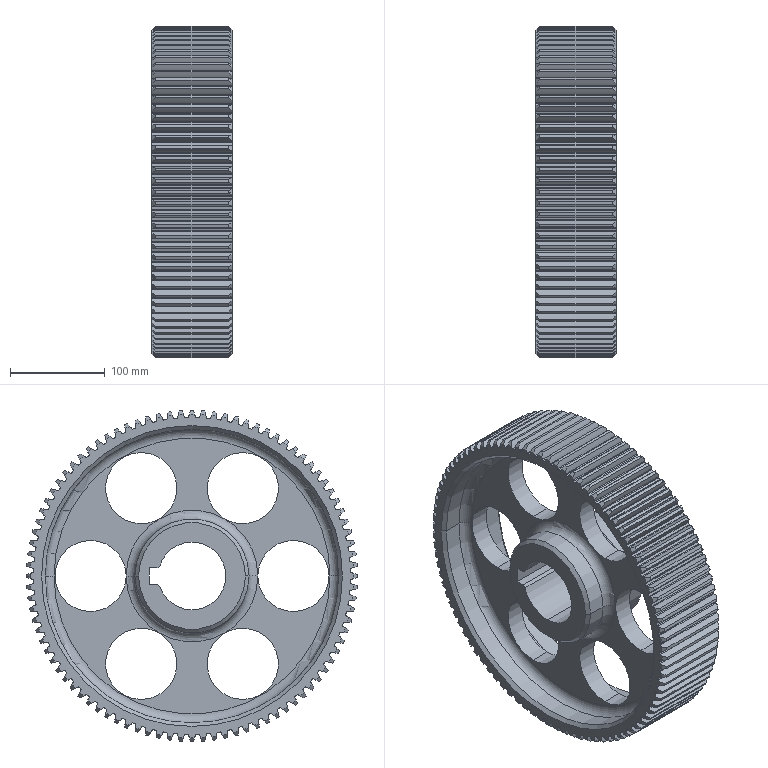Part | SolidWorks | features Chamfer 5, ICE 3, RevCut 1, Revolution 1, Scale 1 | 1 solid | 831 faces | box 84.375 x 348.75 x 348.75 mm | volume 2753310 mm3 | cylinder 618 | cone 194 | plane 11 | torus 8 | commonest cylinder face diameters 1.875 x222 115.716 x188 348.75 x93 333.75 x92 75 x12 120 x4